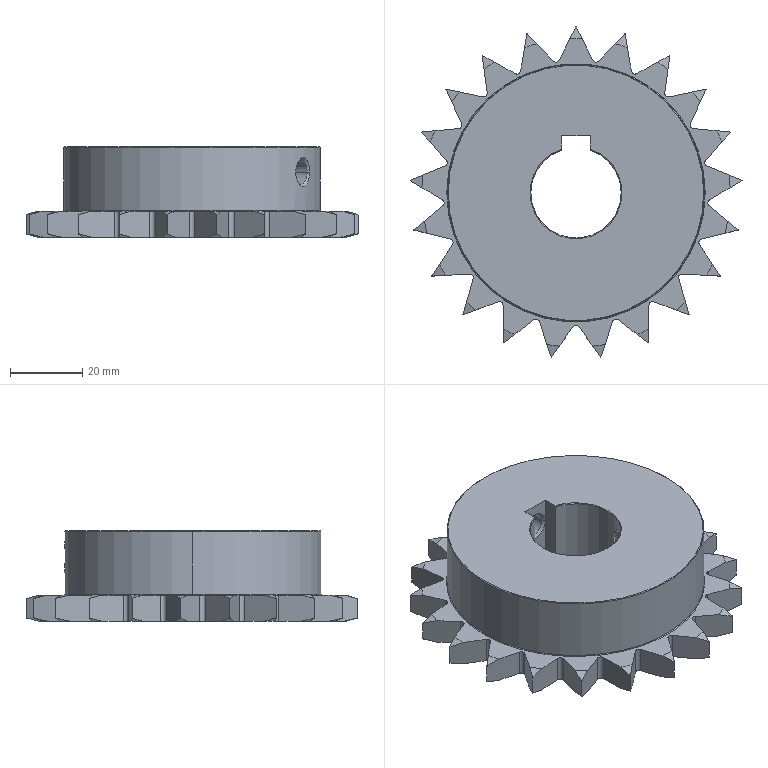Part | STEP file | SP40B21_N_25_SP40B21-N-25 | 1 solid | 190 faces | box 91.743 x 91.486 x 25 mm | volume 93110 mm3 | cone 58 | plane 49 | torus 44 | cylinder 39 | commonest cylinder face diameters 2 x27 6.647 x4 8 x3 25 x3 71 x2